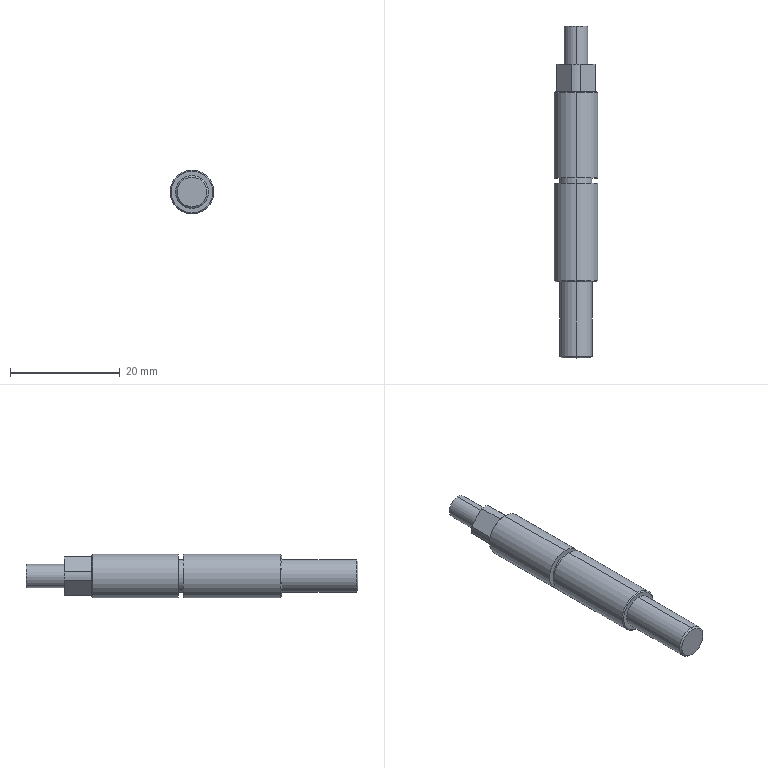Part | SolidWorks | features ICE 3, Chamfer 2, Revolution 1 | 1 solid | 32 faces | box 8 x 60.5 x 8 mm | volume 2374 mm3 | cylinder 15 | plane 11 | cone 6 | commonest cylinder face diameters 7 x5 6 x4 8 x4 4.3 x2
STEP:
#1=CARTESIAN_POINT('',(0.,-43.4,-2.7));
#2=VERTEX_POINT('',#1);
#3=CARTESIAN_POINT('',(0.,-43.4,2.7));
#4=VERTEX_POINT('',#3);
#5=CARTESIAN_POINT('',(0.,-43.4,0.));
#6=DIRECTION('',(0.,-1.,0.));
#7=DIRECTION('',(0.,0.,-1.));
#8=AXIS2_PLACEMENT_3D('',#5,#6,#7);
#9=CIRCLE('',#8,2.7);
#10=EDGE_CURVE('',#2,#4,#9,.T.);
#11=ORIENTED_EDGE('',*,*,#10,.F.);
#12=CARTESIAN_POINT('',(0.,-43.1,-3.));
#13=VERTEX_POINT('',#12);
#14=CARTESIAN_POINT('',(0.,-43.4,-2.7));
#15=DIRECTION('',(0.,0.7071,-0.7071));
#16=VECTOR('',#15,1000.);
#17=LINE('',#14,#16);
#18=EDGE_CURVE('',#2,#13,#17,.T.);
#19=ORIENTED_EDGE('',*,*,#18,.T.);
#20=CARTESIAN_POINT('',(0.,-43.1,3.));
#21=VERTEX_POINT('',#20);
#22=CARTESIAN_POINT('',(0.,-43.1,0.));
#23=DIRECTION('',(0.,1.,0.));
#24=DIRECTION('',(0.,0.,-1.));
#25=AXIS2_PLACEMENT_3D('',#22,#23,#24);
#26=CIRCLE('',#25,3.);
#27=EDGE_CURVE('',#21,#13,#26,.T.);
#28=ORIENTED_EDGE('',*,*,#27,.F.);
#29=CARTESIAN_POINT('',(0.,-43.4,2.7));
#30=DIRECTION('',(0.,0.7071,0.7071));
#31=VECTOR('',#30,1000.);
#32=LINE('',#29,#31);
#33=EDGE_CURVE('',#4,#21,#32,.T.);
#34=ORIENTED_EDGE('',*,*,#33,.F.);
#35=EDGE_LOOP('',(#11,#19,#28,#34));
#36=FACE_OUTER_BOUND('',#35,.T.);
#37=CARTESIAN_POINT('',(0.,-43.4,0.));
#38=DIRECTION('',(0.,1.,0.));
#39=DIRECTION('',(0.,0.,1.));
#40=AXIS2_PLACEMENT_3D('',#37,#38,#39);
#41=CONICAL_SURFACE('',#40,2.7,0.7854);
#42=ADVANCED_FACE('',(#36),#41,.T.);
#43=CARTESIAN_POINT('',(0.,5.1,3.8));
#44=VERTEX_POINT('',#43);
#45=CARTESIAN_POINT('',(0.,5.1,-3.8));
#46=VERTEX_POINT('',#45);
#47=CARTESIAN_POINT('',(0.,5.1,0.));
#48=DIRECTION('',(0.,1.,0.));
#49=DIRECTION('',(0.,0.,1.));
#50=AXIS2_PLACEMENT_3D('',#47,#48,#49);
#51=CIRCLE('',#50,3.8);
#52=EDGE_CURVE('',#44,#46,#51,.T.);
#53=ORIENTED_EDGE('',*,*,#52,.F.);
#54=CARTESIAN_POINT('',(0.,4.9,4.));
#55=VERTEX_POINT('',#54);
#56=CARTESIAN_POINT('',(0.,5.1,3.8));
#57=DIRECTION('',(0.,-0.7071,0.7071));
#58=VECTOR('',#57,1000.);
#59=LINE('',#56,#58);
#60=EDGE_CURVE('',#44,#55,#59,.T.);
#61=ORIENTED_EDGE('',*,*,#60,.T.);
#62=CARTESIAN_POINT('',(0.,4.9,-4.));
#63=VERTEX_POINT('',#62);
#64=CARTESIAN_POINT('',(0.,4.9,0.));
#65=DIRECTION('',(0.,-1.,0.));
#66=DIRECTION('',(0.,0.,1.));
#67=AXIS2_PLACEMENT_3D('',#64,#65,#66);
#68=CIRCLE('',#67,4.);
#69=EDGE_CURVE('',#63,#55,#68,.T.);
#70=ORIENTED_EDGE('',*,*,#69,.F.);
#71=CARTESIAN_POINT('',(0.,5.1,-3.8));
#72=DIRECTION('',(0.,-0.7071,-0.7071));
#73=VECTOR('',#72,1000.);
#74=LINE('',#71,#73);
#75=EDGE_CURVE('',#46,#63,#74,.T.);
#76=ORIENTED_EDGE('',*,*,#75,.F.);
#77=EDGE_LOOP('',(#53,#61,#70,#76));
#78=FACE_OUTER_BOUND('',#77,.T.);
#79=CARTESIAN_POINT('',(0.,5.1,0.));
#80=DIRECTION('',(0.,-1.,0.));
#81=DIRECTION('',(0.,0.,-1.));
#82=AXIS2_PLACEMENT_3D('',#79,#80,#81);
#83=CONICAL_SURFACE('',#82,3.8,0.7854);
#84=ADVANCED_FACE('',(#78),#83,.T.);
#85=CARTESIAN_POINT('',(0.,-29.495,-3.8));
#86=VERTEX_POINT('',#85);
#87=CARTESIAN_POINT('',(0.,-29.495,3.8));
#88=VERTEX_POINT('',#87);
#89=CARTESIAN_POINT('',(0.,-29.495,0.));
#90=DIRECTION('',(0.,-1.,0.));
#91=DIRECTION('',(0.,0.,-1.));
#92=AXIS2_PLACEMENT_3D('',#89,#90,#91);
#93=CIRCLE('',#92,3.8);
#94=EDGE_CURVE('',#86,#88,#93,.T.);
#95=ORIENTED_EDGE('',*,*,#94,.F.);
#96=CARTESIAN_POINT('',(0.,-29.295,-4.));
#97=VERTEX_POINT('',#96);
#98=CARTESIAN_POINT('',(0.,-29.295,-4.));
#99=DIRECTION('',(0.,0.7071,-0.7071));
#100=VECTOR('',#99,1000.);
#101=LINE('',#98,#100);
#102=EDGE_CURVE('',#86,#97,#101,.T.);
#103=ORIENTED_EDGE('',*,*,#102,.T.);
#104=CARTESIAN_POINT('',(0.,-29.295,4.));
#105=VERTEX_POINT('',#104);
#106=CARTESIAN_POINT('',(0.,-29.295,0.));
#107=DIRECTION('',(0.,1.,0.));
#108=DIRECTION('',(0.,0.,-1.));
#109=AXIS2_PLACEMENT_3D('',#106,#107,#108);
#110=CIRCLE('',#109,4.);
#111=EDGE_CURVE('',#105,#97,#110,.T.);
#112=ORIENTED_EDGE('',*,*,#111,.F.);
#113=CARTESIAN_POINT('',(0.,-29.295,4.));
#114=DIRECTION('',(0.,0.7071,0.7071));
#115=VECTOR('',#114,1000.);
#116=LINE('',#113,#115);
#117=EDGE_CURVE('',#88,#105,#116,.T.);
#118=ORIENTED_EDGE('',*,*,#117,.F.);
#119=EDGE_LOOP('',(#95,#103,#112,#118));
#120=FACE_OUTER_BOUND('',#119,.T.);
#121=CARTESIAN_POINT('',(0.,-29.295,0.));
#122=DIRECTION('',(0.,1.,0.));
#123=DIRECTION('',(0.,0.,1.));
#124=AXIS2_PLACEMENT_3D('',#121,#122,#123);
#125=CONICAL_SURFACE('',#124,4.,0.7854);
#126=ADVANCED_FACE('',(#120),#125,.T.);
#127=CARTESIAN_POINT('',(0.,17.1,2.15));
#128=VERTEX_POINT('',#127);
#129=CARTESIAN_POINT('',(0.,17.1,-2.15));
#130=VERTEX_POINT('',#129);
#131=CARTESIAN_POINT('',(0.,17.1,0.));
#132=DIRECTION('',(0.,1.,0.));
#133=DIRECTION('',(0.,0.,1.));
#134=AXIS2_PLACEMENT_3D('',#131,#132,#133);
#135=CIRCLE('',#134,2.15);
#136=EDGE_CURVE('',#128,#130,#135,.T.);
#137=ORIENTED_EDGE('',*,*,#136,.F.);
#138=CARTESIAN_POINT('',(0.,10.1,2.15));
#139=VERTEX_POINT('',#138);
#140=CARTESIAN_POINT('',(0.,17.1,2.15));
#141=DIRECTION('',(0.,-1.,0.));
#142=VECTOR('',#141,1000.);
#143=LINE('',#140,#142);
#144=EDGE_CURVE('',#128,#139,#143,.T.);
#145=ORIENTED_EDGE('',*,*,#144,.T.);
#146=CARTESIAN_POINT('',(0.,10.1,-2.15));
#147=VERTEX_POINT('',#146);
#148=CARTESIAN_POINT('',(0.,10.1,0.));
#149=DIRECTION('',(0.,1.,0.));
#150=DIRECTION('',(0.,0.,1.));
#151=AXIS2_PLACEMENT_3D('',#148,#149,#150);
#152=CIRCLE('',#151,2.15);
#153=EDGE_CURVE('',#139,#147,#152,.T.);
#154=ORIENTED_EDGE('',*,*,#153,.T.);
#155=CARTESIAN_POINT('',(0.,17.1,-2.15));
#156=DIRECTION('',(0.,-1.,0.));
#157=VECTOR('',#156,1000.);
#158=LINE('',#155,#157);
#159=EDGE_CURVE('',#130,#147,#158,.T.);
#160=ORIENTED_EDGE('',*,*,#159,.F.);
#161=EDGE_LOOP('',(#137,#145,#154,#160));
#162=FACE_OUTER_BOUND('',#161,.T.);
#163=CARTESIAN_POINT('',(0.,17.1,0.));
#164=DIRECTION('',(0.,-1.,0.));
#165=DIRECTION('',(0.,0.,-1.));
#166=AXIS2_PLACEMENT_3D('',#163,#164,#165);
#167=CYLINDRICAL_SURFACE('',#166,2.15);
#168=ADVANCED_FACE('',(#162),#167,.T.);
#169=CARTESIAN_POINT('',(0.,10.1,-3.5));
#170=VERTEX_POINT('',#169);
#171=CARTESIAN_POINT('',(-0.7541,10.1,-3.418));
#172=VERTEX_POINT('',#171);
#173=CARTESIAN_POINT('',(0.,10.1,0.));
#174=DIRECTION('',(0.,1.,0.));
#175=DIRECTION('',(0.,0.,-1.));
#176=AXIS2_PLACEMENT_3D('',#173,#174,#175);
#177=CIRCLE('',#176,3.5);
#178=EDGE_CURVE('',#170,#172,#177,.T.);
#179=ORIENTED_EDGE('',*,*,#178,.F.);
#180=CARTESIAN_POINT('',(0.,5.1,-3.5));
#181=VERTEX_POINT('',#180);
#182=CARTESIAN_POINT('',(0.,10.1,-3.5));
#183=DIRECTION('',(0.,-1.,0.));
#184=VECTOR('',#183,1000.);
#185=LINE('',#182,#184);
#186=EDGE_CURVE('',#170,#181,#185,.T.);
#187=ORIENTED_EDGE('',*,*,#186,.T.);
#188=CARTESIAN_POINT('',(-0.7541,5.1,-3.418));
#189=VERTEX_POINT('',#188);
#190=CARTESIAN_POINT('',(0.,5.1,0.));
#191=DIRECTION('',(0.,1.,0.));
#192=DIRECTION('',(0.,0.,-1.));
#193=AXIS2_PLACEMENT_3D('',#190,#191,#192);
#194=CIRCLE('',#193,3.5);
#195=EDGE_CURVE('',#181,#189,#194,.T.);
#196=ORIENTED_EDGE('',*,*,#195,.T.);
#197=CARTESIAN_POINT('',(-0.7541,10.1,-3.418));
#198=DIRECTION('',(0.,-1.,0.));
#199=VECTOR('',#198,1000.);
#200=LINE('',#197,#199);
#201=EDGE_CURVE('',#172,#189,#200,.T.);
#202=ORIENTED_EDGE('',*,*,#201,.F.);
#203=EDGE_LOOP('',(#179,#187,#196,#202));
#204=FACE_OUTER_BOUND('',#203,.T.);
#205=CARTESIAN_POINT('',(0.,10.1,0.));
#206=DIRECTION('',(0.,-1.,0.));
#207=DIRECTION('',(0.,0.,-1.));
#208=AXIS2_PLACEMENT_3D('',#205,#206,#207);
#209=CYLINDRICAL_SURFACE('',#208,3.5);
#210=ADVANCED_FACE('',(#204),#209,.T.);
#211=ORIENTED_EDGE('',*,*,#27,.T.);
#212=CARTESIAN_POINT('',(0.,-29.495,-3.));
#213=VERTEX_POINT('',#212);
#214=CARTESIAN_POINT('',(0.,-43.4,-3.));
#215=DIRECTION('',(0.,1.,0.));
#216=VECTOR('',#215,1000.);
#217=LINE('',#214,#216);
#218=EDGE_CURVE('',#13,#213,#217,.T.);
#219=ORIENTED_EDGE('',*,*,#218,.T.);
#220=CARTESIAN_POINT('',(0.,-29.495,3.));
#221=VERTEX_POINT('',#220);
#222=CARTESIAN_POINT('',(0.,-29.495,0.));
#223=DIRECTION('',(0.,-1.,0.));
#224=DIRECTION('',(0.,0.,-1.));
#225=AXIS2_PLACEMENT_3D('',#222,#223,#224);
#226=CIRCLE('',#225,3.);
#227=EDGE_CURVE('',#213,#221,#226,.T.);
#228=ORIENTED_EDGE('',*,*,#227,.T.);
#229=CARTESIAN_POINT('',(0.,-43.4,3.));
#230=DIRECTION('',(0.,1.,0.));
#231=VECTOR('',#230,1000.);
#232=LINE('',#229,#231);
#233=EDGE_CURVE('',#21,#221,#232,.T.);
#234=ORIENTED_EDGE('',*,*,#233,.F.);
#235=EDGE_LOOP('',(#211,#219,#228,#234));
#236=FACE_OUTER_BOUND('',#235,.T.);
#237=CARTESIAN_POINT('',(0.,-43.4,0.));
#238=DIRECTION('',(0.,1.,0.));
#239=DIRECTION('',(0.,0.,1.));
#240=AXIS2_PLACEMENT_3D('',#237,#238,#239);
#241=CYLINDRICAL_SURFACE('',#240,3.);
#242=ADVANCED_FACE('',(#236),#241,.T.);
#243=CARTESIAN_POINT('',(0.,-11.6,3.));
#244=VERTEX_POINT('',#243);
#245=CARTESIAN_POINT('',(0.,-11.6,-3.));
#246=VERTEX_POINT('',#245);
#247=CARTESIAN_POINT('',(0.,-11.6,0.));
#248=DIRECTION('',(0.,1.,0.));
#249=DIRECTION('',(0.,0.,1.));
#250=AXIS2_PLACEMENT_3D('',#247,#248,#249);
#251=CIRCLE('',#250,3.);
#252=EDGE_CURVE('',#244,#246,#251,.T.);
#253=ORIENTED_EDGE('',*,*,#252,.T.);
#254=CARTESIAN_POINT('',(0.,-10.6,-3.));
#255=VERTEX_POINT('',#254);
#256=CARTESIAN_POINT('',(0.,-29.495,-3.));
#257=DIRECTION('',(0.,1.,0.));
#258=VECTOR('',#257,1000.);
#259=LINE('',#256,#258);
#260=EDGE_CURVE('',#246,#255,#259,.T.);
#261=ORIENTED_EDGE('',*,*,#260,.T.);
#262=CARTESIAN_POINT('',(0.,-10.6,3.));
#263=VERTEX_POINT('',#262);
#264=CARTESIAN_POINT('',(0.,-10.6,0.));
#265=DIRECTION('',(0.,1.,0.));
#266=DIRECTION('',(0.,0.,1.));
#267=AXIS2_PLACEMENT_3D('',#264,#265,#266);
#268=CIRCLE('',#267,3.);
#269=EDGE_CURVE('',#263,#255,#268,.T.);
#270=ORIENTED_EDGE('',*,*,#269,.F.);
#271=CARTESIAN_POINT('',(0.,-29.495,3.));
#272=DIRECTION('',(0.,1.,0.));
#273=VECTOR('',#272,1000.);
#274=LINE('',#271,#273);
#275=EDGE_CURVE('',#244,#263,#274,.T.);
#276=ORIENTED_EDGE('',*,*,#275,.F.);
#277=EDGE_LOOP('',(#253,#261,#270,#276));
#278=FACE_OUTER_BOUND('',#277,.T.);
#279=CARTESIAN_POINT('',(0.,-29.495,0.));
#280=DIRECTION('',(0.,1.,0.));
#281=DIRECTION('',(0.,0.,1.));
#282=AXIS2_PLACEMENT_3D('',#279,#280,#281);
#283=CYLINDRICAL_SURFACE('',#282,3.);
#284=ADVANCED_FACE('',(#278),#283,.T.);
#285=CARTESIAN_POINT('',(0.,-10.6,4.));
#286=VERTEX_POINT('',#285);
#287=CARTESIAN_POINT('',(0.,-10.6,-4.));
#288=VERTEX_POINT('',#287);
#289=CARTESIAN_POINT('',(0.,-10.6,0.));
#290=DIRECTION('',(0.,1.,0.));
#291=DIRECTION('',(0.,0.,1.));
#292=AXIS2_PLACEMENT_3D('',#289,#290,#291);
#293=CIRCLE('',#292,4.);
#294=EDGE_CURVE('',#286,#288,#293,.T.);
#295=ORIENTED_EDGE('',*,*,#294,.T.);
#296=CARTESIAN_POINT('',(0.,-29.495,-4.));
#297=DIRECTION('',(0.,1.,0.));
#298=VECTOR('',#297,1000.);
#299=LINE('',#296,#298);
#300=EDGE_CURVE('',#288,#63,#299,.T.);
#301=ORIENTED_EDGE('',*,*,#300,.T.);
#302=ORIENTED_EDGE('',*,*,#69,.T.);
#303=CARTESIAN_POINT('',(0.,-29.495,4.));
#304=DIRECTION('',(0.,1.,0.));
#305=VECTOR('',#304,1000.);
#306=LINE('',#303,#305);
#307=EDGE_CURVE('',#286,#55,#306,.T.);
#308=ORIENTED_EDGE('',*,*,#307,.F.);
#309=EDGE_LOOP('',(#295,#301,#302,#308));
#310=FACE_OUTER_BOUND('',#309,.T.);
#311=CARTESIAN_POINT('',(0.,-29.495,0.));
#312=DIRECTION('',(0.,1.,0.));
#313=DIRECTION('',(0.,0.,1.));
#314=AXIS2_PLACEMENT_3D('',#311,#312,#313);
#315=CYLINDRICAL_SURFACE('',#314,4.);
#316=ADVANCED_FACE('',(#310),#315,.T.);
#317=ORIENTED_EDGE('',*,*,#111,.T.);
#318=CARTESIAN_POINT('',(0.,-11.6,-4.));
#319=VERTEX_POINT('',#318);
#320=CARTESIAN_POINT('',(0.,-29.495,-4.));
#321=DIRECTION('',(0.,1.,0.));
#322=VECTOR('',#321,1000.);
#323=LINE('',#320,#322);
#324=EDGE_CURVE('',#97,#319,#323,.T.);
#325=ORIENTED_EDGE('',*,*,#324,.T.);
#326=CARTESIAN_POINT('',(0.,-11.6,4.));
#327=VERTEX_POINT('',#326);
#328=CARTESIAN_POINT('',(0.,-11.6,0.));
#329=DIRECTION('',(0.,1.,0.));
#330=DIRECTION('',(0.,0.,1.));
#331=AXIS2_PLACEMENT_3D('',#328,#329,#330);
#332=CIRCLE('',#331,4.);
#333=EDGE_CURVE('',#327,#319,#332,.T.);
#334=ORIENTED_EDGE('',*,*,#333,.F.);
#335=CARTESIAN_POINT('',(0.,-29.495,4.));
#336=DIRECTION('',(0.,1.,0.));
#337=VECTOR('',#336,1000.);
#338=LINE('',#335,#337);
#339=EDGE_CURVE('',#105,#327,#338,.T.);
#340=ORIENTED_EDGE('',*,*,#339,.F.);
#341=EDGE_LOOP('',(#317,#325,#334,#340));
#342=FACE_OUTER_BOUND('',#341,.T.);
#343=CARTESIAN_POINT('',(0.,-29.495,0.));
#344=DIRECTION('',(0.,1.,0.));
#345=DIRECTION('',(0.,0.,1.));
#346=AXIS2_PLACEMENT_3D('',#343,#344,#345);
#347=CYLINDRICAL_SURFACE('',#346,4.);
#348=ADVANCED_FACE('',(#342),#347,.T.);
#349=ORIENTED_EDGE('',*,*,#324,.F.);
#350=CARTESIAN_POINT('',(0.,-29.295,0.));
#351=DIRECTION('',(0.,1.,0.));
#352=DIRECTION('',(0.,0.,-1.));
#353=AXIS2_PLACEMENT_3D('',#350,#351,#352);
#354=CIRCLE('',#353,4.);
#355=EDGE_CURVE('',#97,#105,#354,.T.);
#356=ORIENTED_EDGE('',*,*,#355,.T.);
#357=ORIENTED_EDGE('',*,*,#339,.T.);
#358=CARTESIAN_POINT('',(0.,-11.6,0.));
#359=DIRECTION('',(0.,1.,0.));
#360=DIRECTION('',(0.,0.,1.));
#361=AXIS2_PLACEMENT_3D('',#358,#359,#360);
#362=CIRCLE('',#361,4.);
#363=EDGE_CURVE('',#319,#327,#362,.T.);
#364=ORIENTED_EDGE('',*,*,#363,.F.);
#365=EDGE_LOOP('',(#349,#356,#357,#364));
#366=FACE_OUTER_BOUND('',#365,.T.);
#367=CARTESIAN_POINT('',(0.,-29.495,0.));
#368=DIRECTION('',(0.,1.,0.));
#369=DIRECTION('',(0.,0.,1.));
#370=AXIS2_PLACEMENT_3D('',#367,#368,#369);
#371=CYLINDRICAL_SURFACE('',#370,4.);
#372=ADVANCED_FACE('',(#366),#371,.T.);
#373=CARTESIAN_POINT('',(0.,-29.495,0.));
#374=DIRECTION('',(0.,-1.,0.));
#375=DIRECTION('',(0.,0.,-1.));
#376=AXIS2_PLACEMENT_3D('',#373,#374,#375);
#377=CIRCLE('',#376,3.8);
#378=EDGE_CURVE('',#88,#86,#377,.T.);
#379=ORIENTED_EDGE('',*,*,#378,.T.);
#380=ORIENTED_EDGE('',*,*,#94,.T.);
#381=EDGE_LOOP('',(#379,#380));
#382=FACE_OUTER_BOUND('',#381,.T.);
#383=CARTESIAN_POINT('',(0.,-29.495,0.));
#384=DIRECTION('',(0.,-1.,0.));
#385=DIRECTION('',(0.,0.,-1.));
#386=AXIS2_PLACEMENT_3D('',#383,#384,#385);
#387=CIRCLE('',#386,3.);
#388=EDGE_CURVE('',#221,#213,#387,.T.);
#389=ORIENTED_EDGE('',*,*,#388,.F.);
#390=ORIENTED_EDGE('',*,*,#227,.F.);
#391=EDGE_LOOP('',(#389,#390));
#392=FACE_BOUND('',#391,.T.);
#393=CARTESIAN_POINT('',(4.,-29.495,0.));
#394=DIRECTION('',(0.,-1.,0.));
#395=DIRECTION('',(0.,0.,-1.));
#396=AXIS2_PLACEMENT_3D('',#393,#394,#395);
#397=PLANE('',#396);
#398=ADVANCED_FACE('',(#382,#392),#397,.T.);
#399=CARTESIAN_POINT('',(0.,5.1,0.));
#400=DIRECTION('',(0.,1.,0.));
#401=DIRECTION('',(0.,0.,1.));
#402=AXIS2_PLACEMENT_3D('',#399,#400,#401);
#403=CIRCLE('',#402,3.8);
#404=EDGE_CURVE('',#46,#44,#403,.T.);
#405=ORIENTED_EDGE('',*,*,#404,.T.);
#406=ORIENTED_EDGE('',*,*,#52,.T.);
#407=EDGE_LOOP('',(#405,#406));
#408=FACE_OUTER_BOUND('',#407,.T.);
#409=CARTESIAN_POINT('',(-3.418,5.1,-0.7541));
#410=VERTEX_POINT('',#409);
#411=CARTESIAN_POINT('',(-3.418,5.1,0.7541));
#412=VERTEX_POINT('',#411);
#413=CARTESIAN_POINT('',(0.,5.1,0.));
#414=DIRECTION('',(0.,1.,0.));
#415=DIRECTION('',(0.,0.,-1.));
#416=AXIS2_PLACEMENT_3D('',#413,#414,#415);
#417=CIRCLE('',#416,3.5);
#418=EDGE_CURVE('',#410,#412,#417,.T.);
#419=ORIENTED_EDGE('',*,*,#418,.F.);
#420=CARTESIAN_POINT('',(-3.418,5.1,-0.7541));
#421=DIRECTION('',(-0.7071,0.,0.7071));
#422=VECTOR('',#421,1000.);
#423=LINE('',#420,#422);
#424=EDGE_CURVE('',#189,#410,#423,.T.);
#425=ORIENTED_EDGE('',*,*,#424,.F.);
#426=ORIENTED_EDGE('',*,*,#195,.F.);
#427=CARTESIAN_POINT('',(0.7541,5.1,-3.418));
#428=VERTEX_POINT('',#427);
#429=CARTESIAN_POINT('',(0.,5.1,0.));
#430=DIRECTION('',(0.,1.,0.));
#431=DIRECTION('',(0.,0.,-1.));
#432=AXIS2_PLACEMENT_3D('',#429,#430,#431);
#433=CIRCLE('',#432,3.5);
#434=EDGE_CURVE('',#428,#181,#433,.T.);
#435=ORIENTED_EDGE('',*,*,#434,.F.);
#436=CARTESIAN_POINT('',(3.418,5.1,-0.7541));
#437=VERTEX_POINT('',#436);
#438=CARTESIAN_POINT('',(0.7541,5.1,-3.418));
#439=DIRECTION('',(-0.7071,0.,-0.7071));
#440=VECTOR('',#439,1000.);
#441=LINE('',#438,#440);
#442=EDGE_CURVE('',#437,#428,#441,.T.);
#443=ORIENTED_EDGE('',*,*,#442,.F.);
#444=CARTESIAN_POINT('',(3.418,5.1,0.7541));
#445=VERTEX_POINT('',#444);
#446=CARTESIAN_POINT('',(0.,5.1,0.));
#447=DIRECTION('',(0.,1.,0.));
#448=DIRECTION('',(0.,0.,-1.));
#449=AXIS2_PLACEMENT_3D('',#446,#447,#448);
#450=CIRCLE('',#449,3.5);
#451=EDGE_CURVE('',#445,#437,#450,.T.);
#452=ORIENTED_EDGE('',*,*,#451,.F.);
#453=CARTESIAN_POINT('',(0.7541,5.1,3.418));
#454=VERTEX_POINT('',#453);
#455=CARTESIAN_POINT('',(3.418,5.1,0.7541));
#456=DIRECTION('',(0.7071,0.,-0.7071));
#457=VECTOR('',#456,1000.);
#458=LINE('',#455,#457);
#459=EDGE_CURVE('',#454,#445,#458,.T.);
#460=ORIENTED_EDGE('',*,*,#459,.F.);
#461=CARTESIAN_POINT('',(-0.7541,5.1,3.418));
#462=VERTEX_POINT('',#461);
#463=CARTESIAN_POINT('',(0.,5.1,0.));
#464=DIRECTION('',(0.,1.,0.));
#465=DIRECTION('',(0.,0.,-1.));
#466=AXIS2_PLACEMENT_3D('',#463,#464,#465);
#467=CIRCLE('',#466,3.5);
#468=EDGE_CURVE('',#462,#454,#467,.T.);
#469=ORIENTED_EDGE('',*,*,#468,.F.);
#470=CARTESIAN_POINT('',(-0.7541,5.1,3.418));
#471=DIRECTION('',(0.7071,0.,0.7071));
#472=VECTOR('',#471,1000.);
#473=LINE('',#470,#472);
#474=EDGE_CURVE('',#412,#462,#473,.T.);
#475=ORIENTED_EDGE('',*,*,#474,.F.);
#476=EDGE_LOOP('',(#419,#425,#426,#435,#443,#452,#460,#469,#475));
#477=FACE_BOUND('',#476,.T.);
#478=CARTESIAN_POINT('',(0.,5.1,0.));
#479=DIRECTION('',(0.,1.,0.));
#480=DIRECTION('',(0.,0.,1.));
#481=AXIS2_PLACEMENT_3D('',#478,#479,#480);
#482=PLANE('',#481);
#483=ADVANCED_FACE('',(#408,#477),#482,.T.);
#484=ORIENTED_EDGE('',*,*,#300,.F.);
#485=CARTESIAN_POINT('',(0.,-10.6,0.));
#486=DIRECTION('',(0.,1.,0.));
#487=DIRECTION('',(0.,0.,1.));
#488=AXIS2_PLACEMENT_3D('',#485,#486,#487);
#489=CIRCLE('',#488,4.);
#490=EDGE_CURVE('',#288,#286,#489,.T.);
#491=ORIENTED_EDGE('',*,*,#490,.T.);
#492=ORIENTED_EDGE('',*,*,#307,.T.);
#493=CARTESIAN_POINT('',(0.,4.9,0.));
#494=DIRECTION('',(0.,-1.,0.));
#495=DIRECTION('',(0.,0.,1.));
#496=AXIS2_PLACEMENT_3D('',#493,#494,#495);
#497=CIRCLE('',#496,4.);
#498=EDGE_CURVE('',#55,#63,#497,.T.);
#499=ORIENTED_EDGE('',*,*,#498,.T.);
#500=EDGE_LOOP('',(#484,#491,#492,#499));
#501=FACE_OUTER_BOUND('',#500,.T.);
#502=CARTESIAN_POINT('',(0.,-29.495,0.));
#503=DIRECTION('',(0.,1.,0.));
#504=DIRECTION('',(0.,0.,1.));
#505=AXIS2_PLACEMENT_3D('',#502,#503,#504);
#506=CYLINDRICAL_SURFACE('',#505,4.);
#507=ADVANCED_FACE('',(#501),#506,.T.);
#508=ORIENTED_EDGE('',*,*,#269,.T.);
#509=CARTESIAN_POINT('',(0.,-10.6,0.));
#510=DIRECTION('',(0.,1.,0.));
#511=DIRECTION('',(0.,0.,1.));
#512=AXIS2_PLACEMENT_3D('',#509,#510,#511);
#513=CIRCLE('',#512,3.);
#514=EDGE_CURVE('',#255,#263,#513,.T.);
#515=ORIENTED_EDGE('',*,*,#514,.T.);
#516=EDGE_LOOP('',(#508,#515));
#517=FACE_BOUND('',#516,.T.);
#518=ORIENTED_EDGE('',*,*,#294,.F.);
#519=ORIENTED_EDGE('',*,*,#490,.F.);
#520=EDGE_LOOP('',(#518,#519));
#521=FACE_OUTER_BOUND('',#520,.T.);
#522=CARTESIAN_POINT('',(4.,-10.6,0.));
#523=DIRECTION('',(0.,-1.,0.));
#524=DIRECTION('',(0.,0.,-1.));
#525=AXIS2_PLACEMENT_3D('',#522,#523,#524);
#526=PLANE('',#525);
#527=ADVANCED_FACE('',(#517,#521),#526,.T.);
#528=ORIENTED_EDGE('',*,*,#260,.F.);
#529=CARTESIAN_POINT('',(0.,-11.6,0.));
#530=DIRECTION('',(0.,1.,0.));
#531=DIRECTION('',(0.,0.,1.));
#532=AXIS2_PLACEMENT_3D('',#529,#530,#531);
#533=CIRCLE('',#532,3.);
#534=EDGE_CURVE('',#246,#244,#533,.T.);
#535=ORIENTED_EDGE('',*,*,#534,.T.);
#536=ORIENTED_EDGE('',*,*,#275,.T.);
#537=ORIENTED_EDGE('',*,*,#514,.F.);
#538=EDGE_LOOP('',(#528,#535,#536,#537));
#539=FACE_OUTER_BOUND('',#538,.T.);
#540=CARTESIAN_POINT('',(0.,-29.495,0.));
#541=DIRECTION('',(0.,1.,0.));
#542=DIRECTION('',(0.,0.,1.));
#543=AXIS2_PLACEMENT_3D('',#540,#541,#542);
#544=CYLINDRICAL_SURFACE('',#543,3.);
#545=ADVANCED_FACE('',(#539),#544,.T.);
#546=ORIENTED_EDGE('',*,*,#333,.T.);
#547=ORIENTED_EDGE('',*,*,#363,.T.);
#548=EDGE_LOOP('',(#546,#547));
#549=FACE_OUTER_BOUND('',#548,.T.);
#550=ORIENTED_EDGE('',*,*,#252,.F.);
#551=ORIENTED_EDGE('',*,*,#534,.F.);
#552=EDGE_LOOP('',(#550,#551));
#553=FACE_BOUND('',#552,.T.);
#554=CARTESIAN_POINT('',(3.,-11.6,0.));
#555=DIRECTION('',(0.,1.,0.));
#556=DIRECTION('',(0.,0.,1.));
#557=AXIS2_PLACEMENT_3D('',#554,#555,#556);
#558=PLANE('',#557);
#559=ADVANCED_FACE('',(#549,#553),#558,.T.);
#560=ORIENTED_EDGE('',*,*,#218,.F.);
#561=CARTESIAN_POINT('',(0.,-43.1,0.));
#562=DIRECTION('',(0.,1.,0.));
#563=DIRECTION('',(0.,0.,-1.));
#564=AXIS2_PLACEMENT_3D('',#561,#562,#563);
#565=CIRCLE('',#564,3.);
#566=EDGE_CURVE('',#13,#21,#565,.T.);
#567=ORIENTED_EDGE('',*,*,#566,.T.);
#568=ORIENTED_EDGE('',*,*,#233,.T.);
#569=ORIENTED_EDGE('',*,*,#388,.T.);
#570=EDGE_LOOP('',(#560,#567,#568,#569));
#571=FACE_OUTER_BOUND('',#570,.T.);
#572=CARTESIAN_POINT('',(0.,-43.4,0.));
#573=DIRECTION('',(0.,1.,0.));
#574=DIRECTION('',(0.,0.,1.));
#575=AXIS2_PLACEMENT_3D('',#572,#573,#574);
#576=CYLINDRICAL_SURFACE('',#575,3.);
#577=ADVANCED_FACE('',(#571),#576,.T.);
#578=CARTESIAN_POINT('',(0.,-43.4,0.));
#579=DIRECTION('',(0.,-1.,0.));
#580=DIRECTION('',(0.,0.,-1.));
#581=AXIS2_PLACEMENT_3D('',#578,#579,#580);
#582=CIRCLE('',#581,2.7);
#583=EDGE_CURVE('',#4,#2,#582,.T.);
#584=ORIENTED_EDGE('',*,*,#583,.T.);
#585=ORIENTED_EDGE('',*,*,#10,.T.);
#586=EDGE_LOOP('',(#584,#585));
#587=FACE_OUTER_BOUND('',#586,.T.);
#588=CARTESIAN_POINT('',(0.,-43.4,0.));
#589=DIRECTION('',(0.,-1.,0.));
#590=DIRECTION('',(0.,0.,-1.));
#591=AXIS2_PLACEMENT_3D('',#588,#589,#590);
#592=PLANE('',#591);
#593=ADVANCED_FACE('',(#587),#592,.T.);
#594=ORIENTED_EDGE('',*,*,#418,.T.);
#595=CARTESIAN_POINT('',(-3.418,10.1,0.7541));
#596=VERTEX_POINT('',#595);
#597=CARTESIAN_POINT('',(-3.418,10.1,0.7541));
#598=DIRECTION('',(0.,-1.,0.));
#599=VECTOR('',#598,1000.);
#600=LINE('',#597,#599);
#601=EDGE_CURVE('',#596,#412,#600,.T.);
#602=ORIENTED_EDGE('',*,*,#601,.F.);
#603=CARTESIAN_POINT('',(-3.418,10.1,-0.7541));
#604=VERTEX_POINT('',#603);
#605=CARTESIAN_POINT('',(0.,10.1,0.));
#606=DIRECTION('',(0.,1.,0.));
#607=DIRECTION('',(0.,0.,-1.));
#608=AXIS2_PLACEMENT_3D('',#605,#606,#607);
#609=CIRCLE('',#608,3.5);
#610=EDGE_CURVE('',#604,#596,#609,.T.);
#611=ORIENTED_EDGE('',*,*,#610,.F.);
#612=CARTESIAN_POINT('',(-3.418,10.1,-0.7541));
#613=DIRECTION('',(0.,-1.,0.));
#614=VECTOR('',#613,1000.);
#615=LINE('',#612,#614);
#616=EDGE_CURVE('',#604,#410,#615,.T.);
#617=ORIENTED_EDGE('',*,*,#616,.T.);
#618=EDGE_LOOP('',(#594,#602,#611,#617));
#619=FACE_OUTER_BOUND('',#618,.T.);
#620=CARTESIAN_POINT('',(0.,10.1,0.));
#621=DIRECTION('',(0.,-1.,0.));
#622=DIRECTION('',(0.,0.,-1.));
#623=AXIS2_PLACEMENT_3D('',#620,#621,#622);
#624=CYLINDRICAL_SURFACE('',#623,3.5);
#625=ADVANCED_FACE('',(#619),#624,.T.);
#626=ORIENTED_EDGE('',*,*,#474,.T.);
#627=CARTESIAN_POINT('',(-0.7541,10.1,3.418));
#628=VERTEX_POINT('',#627);
#629=CARTESIAN_POINT('',(-0.7541,10.1,3.418));
#630=DIRECTION('',(0.,-1.,0.));
#631=VECTOR('',#630,1000.);
#632=LINE('',#629,#631);
#633=EDGE_CURVE('',#628,#462,#632,.T.);
#634=ORIENTED_EDGE('',*,*,#633,.F.);
#635=CARTESIAN_POINT('',(-0.7541,10.1,3.418));
#636=DIRECTION('',(0.7071,0.,0.7071));
#637=VECTOR('',#636,1000.);
#638=LINE('',#635,#637);
#639=EDGE_CURVE('',#596,#628,#638,.T.);
#640=ORIENTED_EDGE('',*,*,#639,.F.);
#641=ORIENTED_EDGE('',*,*,#601,.T.);
#642=EDGE_LOOP('',(#626,#634,#640,#641));
#643=FACE_OUTER_BOUND('',#642,.T.);
#644=CARTESIAN_POINT('',(-0.7541,10.1,3.418));
#645=DIRECTION('',(0.7071,0.,-0.7071));
#646=DIRECTION('',(-0.7071,0.,-0.7071));
#647=AXIS2_PLACEMENT_3D('',#644,#645,#646);
#648=PLANE('',#647);
#649=ADVANCED_FACE('',(#643),#648,.F.);
#650=ORIENTED_EDGE('',*,*,#468,.T.);
#651=CARTESIAN_POINT('',(0.7541,10.1,3.418));
#652=VERTEX_POINT('',#651);
#653=CARTESIAN_POINT('',(0.7541,10.1,3.418));
#654=DIRECTION('',(0.,-1.,0.));
#655=VECTOR('',#654,1000.);
#656=LINE('',#653,#655);
#657=EDGE_CURVE('',#652,#454,#656,.T.);
#658=ORIENTED_EDGE('',*,*,#657,.F.);
#659=CARTESIAN_POINT('',(0.,10.1,0.));
#660=DIRECTION('',(0.,1.,0.));
#661=DIRECTION('',(0.,0.,-1.));
#662=AXIS2_PLACEMENT_3D('',#659,#660,#661);
#663=CIRCLE('',#662,3.5);
#664=EDGE_CURVE('',#628,#652,#663,.T.);
#665=ORIENTED_EDGE('',*,*,#664,.F.);
#666=ORIENTED_EDGE('',*,*,#633,.T.);
#667=EDGE_LOOP('',(#650,#658,#665,#666));
#668=FACE_OUTER_BOUND('',#667,.T.);
#669=CARTESIAN_POINT('',(0.,10.1,0.));
#670=DIRECTION('',(0.,-1.,0.));
#671=DIRECTION('',(0.,0.,-1.));
#672=AXIS2_PLACEMENT_3D('',#669,#670,#671);
#673=CYLINDRICAL_SURFACE('',#672,3.5);
#674=ADVANCED_FACE('',(#668),#673,.T.);
#675=ORIENTED_EDGE('',*,*,#459,.T.);
#676=CARTESIAN_POINT('',(3.418,10.1,0.7541));
#677=VERTEX_POINT('',#676);
#678=CARTESIAN_POINT('',(3.418,10.1,0.7541));
#679=DIRECTION('',(0.,-1.,0.));
#680=VECTOR('',#679,1000.);
#681=LINE('',#678,#680);
#682=EDGE_CURVE('',#677,#445,#681,.T.);
#683=ORIENTED_EDGE('',*,*,#682,.F.);
#684=CARTESIAN_POINT('',(3.418,10.1,0.7541));
#685=DIRECTION('',(0.7071,0.,-0.7071));
#686=VECTOR('',#685,1000.);
#687=LINE('',#684,#686);
#688=EDGE_CURVE('',#652,#677,#687,.T.);
#689=ORIENTED_EDGE('',*,*,#688,.F.);
#690=ORIENTED_EDGE('',*,*,#657,.T.);
#691=EDGE_LOOP('',(#675,#683,#689,#690));
#692=FACE_OUTER_BOUND('',#691,.T.);
#693=CARTESIAN_POINT('',(3.418,10.1,0.7541));
#694=DIRECTION('',(-0.7071,0.,-0.7071));
#695=DIRECTION('',(-0.7071,0.,0.7071));
#696=AXIS2_PLACEMENT_3D('',#693,#694,#695);
#697=PLANE('',#696);
#698=ADVANCED_FACE('',(#692),#697,.F.);
#699=ORIENTED_EDGE('',*,*,#451,.T.);
#700=CARTESIAN_POINT('',(3.418,10.1,-0.7541));
#701=VERTEX_POINT('',#700);
#702=CARTESIAN_POINT('',(3.418,10.1,-0.7541));
#703=DIRECTION('',(0.,-1.,0.));
#704=VECTOR('',#703,1000.);
#705=LINE('',#702,#704);
#706=EDGE_CURVE('',#701,#437,#705,.T.);
#707=ORIENTED_EDGE('',*,*,#706,.F.);
#708=CARTESIAN_POINT('',(0.,10.1,0.));
#709=DIRECTION('',(0.,1.,0.));
#710=DIRECTION('',(0.,0.,-1.));
#711=AXIS2_PLACEMENT_3D('',#708,#709,#710);
#712=CIRCLE('',#711,3.5);
#713=EDGE_CURVE('',#677,#701,#712,.T.);
#714=ORIENTED_EDGE('',*,*,#713,.F.);
#715=ORIENTED_EDGE('',*,*,#682,.T.);
#716=EDGE_LOOP('',(#699,#707,#714,#715));
#717=FACE_OUTER_BOUND('',#716,.T.);
#718=CARTESIAN_POINT('',(0.,10.1,0.));
#719=DIRECTION('',(0.,-1.,0.));
#720=DIRECTION('',(0.,0.,-1.));
#721=AXIS2_PLACEMENT_3D('',#718,#719,#720);
#722=CYLINDRICAL_SURFACE('',#721,3.5);
#723=ADVANCED_FACE('',(#717),#722,.T.);
#724=ORIENTED_EDGE('',*,*,#442,.T.);
#725=CARTESIAN_POINT('',(0.7541,10.1,-3.418));
#726=VERTEX_POINT('',#725);
#727=CARTESIAN_POINT('',(0.7541,10.1,-3.418));
#728=DIRECTION('',(0.,-1.,0.));
#729=VECTOR('',#728,1000.);
#730=LINE('',#727,#729);
#731=EDGE_CURVE('',#726,#428,#730,.T.);
#732=ORIENTED_EDGE('',*,*,#731,.F.);
#733=CARTESIAN_POINT('',(0.7541,10.1,-3.418));
#734=DIRECTION('',(-0.7071,0.,-0.7071));
#735=VECTOR('',#734,1000.);
#736=LINE('',#733,#735);
#737=EDGE_CURVE('',#701,#726,#736,.T.);
#738=ORIENTED_EDGE('',*,*,#737,.F.);
#739=ORIENTED_EDGE('',*,*,#706,.T.);
#740=EDGE_LOOP('',(#724,#732,#738,#739));
#741=FACE_OUTER_BOUND('',#740,.T.);
#742=CARTESIAN_POINT('',(0.7541,10.1,-3.418));
#743=DIRECTION('',(-0.7071,0.,0.7071));
#744=DIRECTION('',(0.7071,0.,0.7071));
#745=AXIS2_PLACEMENT_3D('',#742,#743,#744);
#746=PLANE('',#745);
#747=ADVANCED_FACE('',(#741),#746,.F.);
#748=ORIENTED_EDGE('',*,*,#186,.F.);
#749=CARTESIAN_POINT('',(0.,10.1,0.));
#750=DIRECTION('',(0.,1.,0.));
#751=DIRECTION('',(0.,0.,-1.));
#752=AXIS2_PLACEMENT_3D('',#749,#750,#751);
#753=CIRCLE('',#752,3.5);
#754=EDGE_CURVE('',#726,#170,#753,.T.);
#755=ORIENTED_EDGE('',*,*,#754,.F.);
#756=ORIENTED_EDGE('',*,*,#731,.T.);
#757=ORIENTED_EDGE('',*,*,#434,.T.);
#758=EDGE_LOOP('',(#748,#755,#756,#757));
#759=FACE_OUTER_BOUND('',#758,.T.);
#760=CARTESIAN_POINT('',(0.,10.1,0.));
#761=DIRECTION('',(0.,-1.,0.));
#762=DIRECTION('',(0.,0.,-1.));
#763=AXIS2_PLACEMENT_3D('',#760,#761,#762);
#764=CYLINDRICAL_SURFACE('',#763,3.5);
#765=ADVANCED_FACE('',(#759),#764,.T.);
#766=ORIENTED_EDGE('',*,*,#424,.T.);
#767=ORIENTED_EDGE('',*,*,#616,.F.);
#768=CARTESIAN_POINT('',(-3.418,10.1,-0.7541));
#769=DIRECTION('',(-0.7071,0.,0.7071));
#770=VECTOR('',#769,1000.);
#771=LINE('',#768,#770);
#772=EDGE_CURVE('',#172,#604,#771,.T.);
#773=ORIENTED_EDGE('',*,*,#772,.F.);
#774=ORIENTED_EDGE('',*,*,#201,.T.);
#775=EDGE_LOOP('',(#766,#767,#773,#774));
#776=FACE_OUTER_BOUND('',#775,.T.);
#777=CARTESIAN_POINT('',(-3.418,10.1,-0.7541));
#778=DIRECTION('',(0.7071,0.,0.7071));
#779=DIRECTION('',(0.7071,0.,-0.7071));
#780=AXIS2_PLACEMENT_3D('',#777,#778,#779);
#781=PLANE('',#780);
#782=ADVANCED_FACE('',(#776),#781,.F.);
#783=CARTESIAN_POINT('',(0.,10.1,0.));
#784=DIRECTION('',(0.,1.,0.));
#785=DIRECTION('',(0.,0.,1.));
#786=AXIS2_PLACEMENT_3D('',#783,#784,#785);
#787=CIRCLE('',#786,2.15);
#788=EDGE_CURVE('',#147,#139,#787,.T.);
#789=ORIENTED_EDGE('',*,*,#788,.F.);
#790=ORIENTED_EDGE('',*,*,#153,.F.);
#791=EDGE_LOOP('',(#789,#790));
#792=FACE_BOUND('',#791,.T.);
#793=ORIENTED_EDGE('',*,*,#610,.T.);
#794=ORIENTED_EDGE('',*,*,#639,.T.);
#795=ORIENTED_EDGE('',*,*,#664,.T.);
#796=ORIENTED_EDGE('',*,*,#688,.T.);
#797=ORIENTED_EDGE('',*,*,#713,.T.);
#798=ORIENTED_EDGE('',*,*,#737,.T.);
#799=ORIENTED_EDGE('',*,*,#754,.T.);
#800=ORIENTED_EDGE('',*,*,#178,.T.);
#801=ORIENTED_EDGE('',*,*,#772,.T.);
#802=EDGE_LOOP('',(#793,#794,#795,#796,#797,#798,#799,#800,#801));
#803=FACE_OUTER_BOUND('',#802,.T.);
#804=CARTESIAN_POINT('',(0.,10.1,0.));
#805=DIRECTION('',(0.,-1.,0.));
#806=DIRECTION('',(0.,0.,-1.));
#807=AXIS2_PLACEMENT_3D('',#804,#805,#806);
#808=PLANE('',#807);
#809=ADVANCED_FACE('',(#792,#803),#808,.F.);
#810=ORIENTED_EDGE('',*,*,#144,.F.);
#811=CARTESIAN_POINT('',(0.,17.1,0.));
#812=DIRECTION('',(0.,1.,0.));
#813=DIRECTION('',(0.,0.,1.));
#814=AXIS2_PLACEMENT_3D('',#811,#812,#813);
#815=CIRCLE('',#814,2.15);
#816=EDGE_CURVE('',#130,#128,#815,.T.);
#817=ORIENTED_EDGE('',*,*,#816,.F.);
#818=ORIENTED_EDGE('',*,*,#159,.T.);
#819=ORIENTED_EDGE('',*,*,#788,.T.);
#820=EDGE_LOOP('',(#810,#817,#818,#819));
#821=FACE_OUTER_BOUND('',#820,.T.);
#822=CARTESIAN_POINT('',(0.,17.1,0.));
#823=DIRECTION('',(0.,-1.,0.));
#824=DIRECTION('',(0.,0.,-1.));
#825=AXIS2_PLACEMENT_3D('',#822,#823,#824);
#826=CYLINDRICAL_SURFACE('',#825,2.15);
#827=ADVANCED_FACE('',(#821),#826,.T.);
#828=ORIENTED_EDGE('',*,*,#816,.T.);
#829=ORIENTED_EDGE('',*,*,#136,.T.);
#830=EDGE_LOOP('',(#828,#829));
#831=FACE_OUTER_BOUND('',#830,.T.);
#832=CARTESIAN_POINT('',(0.,17.1,0.));
#833=DIRECTION('',(0.,1.,0.));
#834=DIRECTION('',(0.,0.,1.));
#835=AXIS2_PLACEMENT_3D('',#832,#833,#834);
#836=PLANE('',#835);
#837=ADVANCED_FACE('',(#831),#836,.T.);
#838=ORIENTED_EDGE('',*,*,#102,.F.);
#839=ORIENTED_EDGE('',*,*,#378,.F.);
#840=ORIENTED_EDGE('',*,*,#117,.T.);
#841=ORIENTED_EDGE('',*,*,#355,.F.);
#842=EDGE_LOOP('',(#838,#839,#840,#841));
#843=FACE_OUTER_BOUND('',#842,.T.);
#844=CARTESIAN_POINT('',(0.,-29.295,0.));
#845=DIRECTION('',(0.,1.,0.));
#846=DIRECTION('',(0.,0.,1.));
#847=AXIS2_PLACEMENT_3D('',#844,#845,#846);
#848=CONICAL_SURFACE('',#847,4.,0.7854);
#849=ADVANCED_FACE('',(#843),#848,.T.);
#850=ORIENTED_EDGE('',*,*,#60,.F.);
#851=ORIENTED_EDGE('',*,*,#404,.F.);
#852=ORIENTED_EDGE('',*,*,#75,.T.);
#853=ORIENTED_EDGE('',*,*,#498,.F.);
#854=EDGE_LOOP('',(#850,#851,#852,#853));
#855=FACE_OUTER_BOUND('',#854,.T.);
#856=CARTESIAN_POINT('',(0.,5.1,0.));
#857=DIRECTION('',(0.,-1.,0.));
#858=DIRECTION('',(0.,0.,-1.));
#859=AXIS2_PLACEMENT_3D('',#856,#857,#858);
#860=CONICAL_SURFACE('',#859,3.8,0.7854);
#861=ADVANCED_FACE('',(#855),#860,.T.);
#862=ORIENTED_EDGE('',*,*,#18,.F.);
#863=ORIENTED_EDGE('',*,*,#583,.F.);
#864=ORIENTED_EDGE('',*,*,#33,.T.);
#865=ORIENTED_EDGE('',*,*,#566,.F.);
#866=EDGE_LOOP('',(#862,#863,#864,#865));
#867=FACE_OUTER_BOUND('',#866,.T.);
#868=CARTESIAN_POINT('',(0.,-43.4,0.));
#869=DIRECTION('',(0.,1.,0.));
#870=DIRECTION('',(0.,0.,1.));
#871=AXIS2_PLACEMENT_3D('',#868,#869,#870);
#872=CONICAL_SURFACE('',#871,2.7,0.7854);
#873=ADVANCED_FACE('',(#867),#872,.T.);
#874=CLOSED_SHELL('',(#42,#84,#126,#168,#210,#242,#284,#316,#348,#372,#398,#483,#507,#527,#545,#559,#577,#593,#625,#649,#674,#698,#723,#747,#765,#782,#809,#827,#837,#849,#861,#873));
#875=MANIFOLD_SOLID_BREP('',#874);
#876=CARTESIAN_POINT('',(0.,0.,0.));
#877=DIRECTION('',(0.,0.,1.));
#878=DIRECTION('',(1.,0.,0.));
#879=AXIS2_PLACEMENT_3D('',#876,#877,#878);
#880=(LENGTH_UNIT()NAMED_UNIT(*)SI_UNIT(.MILLI.,.METRE.));
#881=UNCERTAINTY_MEASURE_WITH_UNIT(LENGTH_MEASURE(0.00001),#880,'','');
#882=(NAMED_UNIT(*)PLANE_ANGLE_UNIT()SI_UNIT($,.RADIAN.));
#883=(NAMED_UNIT(*)SI_UNIT($,.STERADIAN.)SOLID_ANGLE_UNIT());
#884=(GEOMETRIC_REPRESENTATION_CONTEXT(3)GLOBAL_UNCERTAINTY_ASSIGNED_CONTEXT((#881))GLOBAL_UNIT_ASSIGNED_CONTEXT((#880,#882,#883))REPRESENTATION_CONTEXT('',''));
#885=ADVANCED_BREP_SHAPE_REPRESENTATION('',(#875,#879),#884);